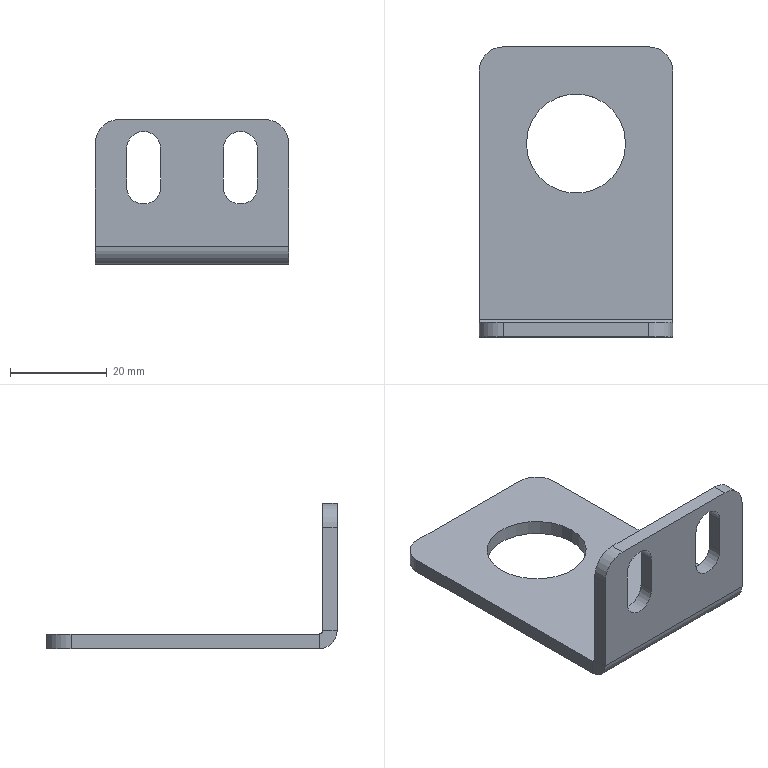Part | SolidWorks | features BaseBody 1 | 1 solid | 30 faces | box 40 x 60 x 30 mm | volume 8703 mm3 | plane 16 | cylinder 14 | commonest cylinder face diameters 7 x6 10 x4 20.5 x2 1.473 x1 7.473 x1
STEP:
#1=CARTESIAN_POINT('',(10.,-31.5,24.5));
#2=VERTEX_POINT('',#1);
#3=CARTESIAN_POINT('',(13.5,-31.5,21.));
#4=VERTEX_POINT('',#3);
#5=CARTESIAN_POINT('',(10.,-31.5,21.));
#6=DIRECTION('',(0.,1.,0.));
#7=DIRECTION('',(0.,0.,1.));
#8=AXIS2_PLACEMENT_3D('',#5,#6,#7);
#9=CIRCLE('',#8,3.5);
#10=EDGE_CURVE('',#2,#4,#9,.T.);
#11=ORIENTED_EDGE('',*,*,#10,.F.);
#12=CARTESIAN_POINT('',(10.,-28.5,24.5));
#13=VERTEX_POINT('',#12);
#14=CARTESIAN_POINT('',(10.,-38.5,24.5));
#15=DIRECTION('',(0.,1.,0.));
#16=VECTOR('',#15,1000.);
#17=LINE('',#14,#16);
#18=EDGE_CURVE('',#2,#13,#17,.T.);
#19=ORIENTED_EDGE('',*,*,#18,.T.);
#20=CARTESIAN_POINT('',(13.5,-28.5,21.));
#21=VERTEX_POINT('',#20);
#22=CARTESIAN_POINT('',(10.,-28.5,21.));
#23=DIRECTION('',(0.,1.,0.));
#24=DIRECTION('',(0.,0.,1.));
#25=AXIS2_PLACEMENT_3D('',#22,#23,#24);
#26=CIRCLE('',#25,3.5);
#27=EDGE_CURVE('',#13,#21,#26,.T.);
#28=ORIENTED_EDGE('',*,*,#27,.T.);
#29=CARTESIAN_POINT('',(13.5,-38.5,21.));
#30=DIRECTION('',(0.,1.,0.));
#31=VECTOR('',#30,1000.);
#32=LINE('',#29,#31);
#33=EDGE_CURVE('',#4,#21,#32,.T.);
#34=ORIENTED_EDGE('',*,*,#33,.F.);
#35=EDGE_LOOP('',(#11,#19,#28,#34));
#36=FACE_OUTER_BOUND('',#35,.T.);
#37=CARTESIAN_POINT('',(10.,-38.5,21.));
#38=DIRECTION('',(0.,1.,0.));
#39=DIRECTION('',(0.,0.,1.));
#40=AXIS2_PLACEMENT_3D('',#37,#38,#39);
#41=CYLINDRICAL_SURFACE('',#40,3.5);
#42=ADVANCED_FACE('',(#36),#41,.F.);
#43=CARTESIAN_POINT('',(-10.,-31.5,24.5));
#44=VERTEX_POINT('',#43);
#45=CARTESIAN_POINT('',(-6.5,-31.5,21.));
#46=VERTEX_POINT('',#45);
#47=CARTESIAN_POINT('',(-10.,-31.5,21.));
#48=DIRECTION('',(0.,1.,0.));
#49=DIRECTION('',(0.,0.,1.));
#50=AXIS2_PLACEMENT_3D('',#47,#48,#49);
#51=CIRCLE('',#50,3.5);
#52=EDGE_CURVE('',#44,#46,#51,.T.);
#53=ORIENTED_EDGE('',*,*,#52,.F.);
#54=CARTESIAN_POINT('',(-10.,-28.5,24.5));
#55=VERTEX_POINT('',#54);
#56=CARTESIAN_POINT('',(-10.,-38.5,24.5));
#57=DIRECTION('',(0.,1.,0.));
#58=VECTOR('',#57,1000.);
#59=LINE('',#56,#58);
#60=EDGE_CURVE('',#44,#55,#59,.T.);
#61=ORIENTED_EDGE('',*,*,#60,.T.);
#62=CARTESIAN_POINT('',(-6.5,-28.5,21.));
#63=VERTEX_POINT('',#62);
#64=CARTESIAN_POINT('',(-10.,-28.5,21.));
#65=DIRECTION('',(0.,1.,0.));
#66=DIRECTION('',(0.,0.,1.));
#67=AXIS2_PLACEMENT_3D('',#64,#65,#66);
#68=CIRCLE('',#67,3.5);
#69=EDGE_CURVE('',#55,#63,#68,.T.);
#70=ORIENTED_EDGE('',*,*,#69,.T.);
#71=CARTESIAN_POINT('',(-6.5,-38.5,21.));
#72=DIRECTION('',(0.,1.,0.));
#73=VECTOR('',#72,1000.);
#74=LINE('',#71,#73);
#75=EDGE_CURVE('',#46,#63,#74,.T.);
#76=ORIENTED_EDGE('',*,*,#75,.F.);
#77=EDGE_LOOP('',(#53,#61,#70,#76));
#78=FACE_OUTER_BOUND('',#77,.T.);
#79=CARTESIAN_POINT('',(-10.,-38.5,21.));
#80=DIRECTION('',(0.,1.,0.));
#81=DIRECTION('',(0.,0.,1.));
#82=AXIS2_PLACEMENT_3D('',#79,#80,#81);
#83=CYLINDRICAL_SURFACE('',#82,3.5);
#84=ADVANCED_FACE('',(#78),#83,.F.);
#85=CARTESIAN_POINT('',(-10.25,8.5,0.));
#86=VERTEX_POINT('',#85);
#87=CARTESIAN_POINT('',(10.25,8.5,0.));
#88=VERTEX_POINT('',#87);
#89=CARTESIAN_POINT('',(0.,8.5,0.));
#90=DIRECTION('',(0.,0.,1.));
#91=DIRECTION('',(1.,0.,0.));
#92=AXIS2_PLACEMENT_3D('',#89,#90,#91);
#93=CIRCLE('',#92,10.25);
#94=EDGE_CURVE('',#86,#88,#93,.T.);
#95=ORIENTED_EDGE('',*,*,#94,.T.);
#96=CARTESIAN_POINT('',(10.25,8.5,-3.));
#97=VERTEX_POINT('',#96);
#98=CARTESIAN_POINT('',(10.25,8.5,-3.));
#99=DIRECTION('',(0.,0.,-1.));
#100=VECTOR('',#99,1000.);
#101=LINE('',#98,#100);
#102=EDGE_CURVE('',#88,#97,#101,.T.);
#103=ORIENTED_EDGE('',*,*,#102,.T.);
#104=CARTESIAN_POINT('',(-10.25,8.5,-3.));
#105=VERTEX_POINT('',#104);
#106=CARTESIAN_POINT('',(0.,8.5,-3.));
#107=DIRECTION('',(0.,0.,-1.));
#108=DIRECTION('',(-1.,0.,0.));
#109=AXIS2_PLACEMENT_3D('',#106,#107,#108);
#110=CIRCLE('',#109,10.25);
#111=EDGE_CURVE('',#97,#105,#110,.T.);
#112=ORIENTED_EDGE('',*,*,#111,.T.);
#113=CARTESIAN_POINT('',(-10.25,8.5,-3.));
#114=DIRECTION('',(0.,0.,-1.));
#115=VECTOR('',#114,1000.);
#116=LINE('',#113,#115);
#117=EDGE_CURVE('',#86,#105,#116,.T.);
#118=ORIENTED_EDGE('',*,*,#117,.F.);
#119=EDGE_LOOP('',(#95,#103,#112,#118));
#120=FACE_OUTER_BOUND('',#119,.T.);
#121=CARTESIAN_POINT('',(0.,8.5,-3.));
#122=DIRECTION('',(0.,0.,-1.));
#123=DIRECTION('',(-1.,0.,0.));
#124=AXIS2_PLACEMENT_3D('',#121,#122,#123);
#125=CYLINDRICAL_SURFACE('',#124,10.25);
#126=ADVANCED_FACE('',(#120),#125,.F.);
#127=CARTESIAN_POINT('',(20.,-27.763,-3.));
#128=VERTEX_POINT('',#127);
#129=CARTESIAN_POINT('',(20.,23.5,-3.));
#130=VERTEX_POINT('',#129);
#131=CARTESIAN_POINT('',(20.,28.5,-3.));
#132=DIRECTION('',(0.,1.,0.));
#133=VECTOR('',#132,1000.);
#134=LINE('',#131,#133);
#135=EDGE_CURVE('',#128,#130,#134,.T.);
#136=ORIENTED_EDGE('',*,*,#135,.T.);
#137=CARTESIAN_POINT('',(20.,23.5,0.));
#138=VERTEX_POINT('',#137);
#139=CARTESIAN_POINT('',(20.,23.5,-3.));
#140=DIRECTION('',(0.,0.,1.));
#141=VECTOR('',#140,1000.);
#142=LINE('',#139,#141);
#143=EDGE_CURVE('',#130,#138,#142,.T.);
#144=ORIENTED_EDGE('',*,*,#143,.T.);
#145=CARTESIAN_POINT('',(20.,-27.763,0.));
#146=VERTEX_POINT('',#145);
#147=CARTESIAN_POINT('',(20.,28.5,0.));
#148=DIRECTION('',(0.,1.,0.));
#149=VECTOR('',#148,1000.);
#150=LINE('',#147,#149);
#151=EDGE_CURVE('',#146,#138,#150,.T.);
#152=ORIENTED_EDGE('',*,*,#151,.F.);
#153=CARTESIAN_POINT('',(20.,-27.763,0.));
#154=DIRECTION('',(0.,0.,-1.));
#155=VECTOR('',#154,1000.);
#156=LINE('',#153,#155);
#157=EDGE_CURVE('',#146,#128,#156,.T.);
#158=ORIENTED_EDGE('',*,*,#157,.T.);
#159=EDGE_LOOP('',(#136,#144,#152,#158));
#160=FACE_OUTER_BOUND('',#159,.T.);
#161=CARTESIAN_POINT('',(20.,28.5,-3.));
#162=DIRECTION('',(1.,0.,0.));
#163=DIRECTION('',(0.,1.,0.));
#164=AXIS2_PLACEMENT_3D('',#161,#162,#163);
#165=PLANE('',#164);
#166=ADVANCED_FACE('',(#160),#165,.T.);
#167=CARTESIAN_POINT('',(0.,8.5,-3.));
#168=DIRECTION('',(0.,0.,-1.));
#169=DIRECTION('',(-1.,0.,0.));
#170=AXIS2_PLACEMENT_3D('',#167,#168,#169);
#171=CIRCLE('',#170,10.25);
#172=EDGE_CURVE('',#105,#97,#171,.T.);
#173=ORIENTED_EDGE('',*,*,#172,.F.);
#174=ORIENTED_EDGE('',*,*,#111,.F.);
#175=EDGE_LOOP('',(#173,#174));
#176=FACE_BOUND('',#175,.T.);
#177=CARTESIAN_POINT('',(15.,28.5,-3.));
#178=VERTEX_POINT('',#177);
#179=CARTESIAN_POINT('',(-15.,28.5,-3.));
#180=VERTEX_POINT('',#179);
#181=CARTESIAN_POINT('',(-20.,28.5,-3.));
#182=DIRECTION('',(-1.,0.,0.));
#183=VECTOR('',#182,1000.);
#184=LINE('',#181,#183);
#185=EDGE_CURVE('',#178,#180,#184,.T.);
#186=ORIENTED_EDGE('',*,*,#185,.F.);
#187=CARTESIAN_POINT('',(15.,23.5,-3.));
#188=DIRECTION('',(0.,0.,-1.));
#189=DIRECTION('',(1.,0.,0.));
#190=AXIS2_PLACEMENT_3D('',#187,#188,#189);
#191=CIRCLE('',#190,5.);
#192=EDGE_CURVE('',#178,#130,#191,.T.);
#193=ORIENTED_EDGE('',*,*,#192,.T.);
#194=ORIENTED_EDGE('',*,*,#135,.F.);
#195=CARTESIAN_POINT('',(-20.,-27.763,-3.));
#196=VERTEX_POINT('',#195);
#197=CARTESIAN_POINT('',(20.,-27.763,-3.));
#198=DIRECTION('',(-1.,0.,0.));
#199=VECTOR('',#198,1000.);
#200=LINE('',#197,#199);
#201=EDGE_CURVE('',#128,#196,#200,.T.);
#202=ORIENTED_EDGE('',*,*,#201,.T.);
#203=CARTESIAN_POINT('',(-20.,23.5,-3.));
#204=VERTEX_POINT('',#203);
#205=CARTESIAN_POINT('',(-20.,28.5,-3.));
#206=DIRECTION('',(0.,-1.,0.));
#207=VECTOR('',#206,1000.);
#208=LINE('',#205,#207);
#209=EDGE_CURVE('',#204,#196,#208,.T.);
#210=ORIENTED_EDGE('',*,*,#209,.F.);
#211=CARTESIAN_POINT('',(-15.,23.5,-3.));
#212=DIRECTION('',(0.,0.,-1.));
#213=DIRECTION('',(1.,0.,0.));
#214=AXIS2_PLACEMENT_3D('',#211,#212,#213);
#215=CIRCLE('',#214,5.);
#216=EDGE_CURVE('',#204,#180,#215,.T.);
#217=ORIENTED_EDGE('',*,*,#216,.T.);
#218=EDGE_LOOP('',(#186,#193,#194,#202,#210,#217));
#219=FACE_OUTER_BOUND('',#218,.T.);
#220=CARTESIAN_POINT('',(0.,0.,-3.));
#221=DIRECTION('',(0.,0.,1.));
#222=DIRECTION('',(1.,0.,0.));
#223=AXIS2_PLACEMENT_3D('',#220,#221,#222);
#224=PLANE('',#223);
#225=ADVANCED_FACE('',(#176,#219),#224,.F.);
#226=ORIENTED_EDGE('',*,*,#94,.F.);
#227=CARTESIAN_POINT('',(0.,8.5,0.));
#228=DIRECTION('',(0.,0.,1.));
#229=DIRECTION('',(1.,0.,0.));
#230=AXIS2_PLACEMENT_3D('',#227,#228,#229);
#231=CIRCLE('',#230,10.25);
#232=EDGE_CURVE('',#88,#86,#231,.T.);
#233=ORIENTED_EDGE('',*,*,#232,.F.);
#234=EDGE_LOOP('',(#226,#233));
#235=FACE_BOUND('',#234,.T.);
#236=ORIENTED_EDGE('',*,*,#151,.T.);
#237=CARTESIAN_POINT('',(15.,28.5,0.));
#238=VERTEX_POINT('',#237);
#239=CARTESIAN_POINT('',(15.,23.5,0.));
#240=DIRECTION('',(0.,0.,1.));
#241=DIRECTION('',(1.,0.,0.));
#242=AXIS2_PLACEMENT_3D('',#239,#240,#241);
#243=CIRCLE('',#242,5.);
#244=EDGE_CURVE('',#138,#238,#243,.T.);
#245=ORIENTED_EDGE('',*,*,#244,.T.);
#246=CARTESIAN_POINT('',(-15.,28.5,0.));
#247=VERTEX_POINT('',#246);
#248=CARTESIAN_POINT('',(-20.,28.5,0.));
#249=DIRECTION('',(-1.,0.,0.));
#250=VECTOR('',#249,1000.);
#251=LINE('',#248,#250);
#252=EDGE_CURVE('',#238,#247,#251,.T.);
#253=ORIENTED_EDGE('',*,*,#252,.T.);
#254=CARTESIAN_POINT('',(-20.,23.5,0.));
#255=VERTEX_POINT('',#254);
#256=CARTESIAN_POINT('',(-15.,23.5,0.));
#257=DIRECTION('',(0.,0.,1.));
#258=DIRECTION('',(1.,0.,0.));
#259=AXIS2_PLACEMENT_3D('',#256,#257,#258);
#260=CIRCLE('',#259,5.);
#261=EDGE_CURVE('',#247,#255,#260,.T.);
#262=ORIENTED_EDGE('',*,*,#261,.T.);
#263=CARTESIAN_POINT('',(-20.,-27.763,0.));
#264=VERTEX_POINT('',#263);
#265=CARTESIAN_POINT('',(-20.,28.5,0.));
#266=DIRECTION('',(0.,-1.,0.));
#267=VECTOR('',#266,1000.);
#268=LINE('',#265,#267);
#269=EDGE_CURVE('',#255,#264,#268,.T.);
#270=ORIENTED_EDGE('',*,*,#269,.T.);
#271=CARTESIAN_POINT('',(20.,-27.763,0.));
#272=DIRECTION('',(-1.,0.,0.));
#273=VECTOR('',#272,1000.);
#274=LINE('',#271,#273);
#275=EDGE_CURVE('',#146,#264,#274,.T.);
#276=ORIENTED_EDGE('',*,*,#275,.F.);
#277=EDGE_LOOP('',(#236,#245,#253,#262,#270,#276));
#278=FACE_OUTER_BOUND('',#277,.T.);
#279=CARTESIAN_POINT('',(0.,0.,0.));
#280=DIRECTION('',(0.,0.,1.));
#281=DIRECTION('',(1.,0.,0.));
#282=AXIS2_PLACEMENT_3D('',#279,#280,#281);
#283=PLANE('',#282);
#284=ADVANCED_FACE('',(#235,#278),#283,.T.);
#285=ORIENTED_EDGE('',*,*,#269,.F.);
#286=CARTESIAN_POINT('',(-20.,23.5,-3.));
#287=DIRECTION('',(0.,0.,-1.));
#288=VECTOR('',#287,1000.);
#289=LINE('',#286,#288);
#290=EDGE_CURVE('',#255,#204,#289,.T.);
#291=ORIENTED_EDGE('',*,*,#290,.T.);
#292=ORIENTED_EDGE('',*,*,#209,.T.);
#293=CARTESIAN_POINT('',(-20.,-27.763,0.));
#294=DIRECTION('',(0.,0.,-1.));
#295=VECTOR('',#294,1000.);
#296=LINE('',#293,#295);
#297=EDGE_CURVE('',#264,#196,#296,.T.);
#298=ORIENTED_EDGE('',*,*,#297,.F.);
#299=EDGE_LOOP('',(#285,#291,#292,#298));
#300=FACE_OUTER_BOUND('',#299,.T.);
#301=CARTESIAN_POINT('',(-20.,28.5,-3.));
#302=DIRECTION('',(-1.,0.,0.));
#303=DIRECTION('',(0.,-1.,0.));
#304=AXIS2_PLACEMENT_3D('',#301,#302,#303);
#305=PLANE('',#304);
#306=ADVANCED_FACE('',(#300),#305,.T.);
#307=ORIENTED_EDGE('',*,*,#252,.F.);
#308=CARTESIAN_POINT('',(15.,28.5,-3.));
#309=DIRECTION('',(0.,0.,-1.));
#310=VECTOR('',#309,1000.);
#311=LINE('',#308,#310);
#312=EDGE_CURVE('',#238,#178,#311,.T.);
#313=ORIENTED_EDGE('',*,*,#312,.T.);
#314=ORIENTED_EDGE('',*,*,#185,.T.);
#315=CARTESIAN_POINT('',(-15.,28.5,-3.));
#316=DIRECTION('',(0.,0.,1.));
#317=VECTOR('',#316,1000.);
#318=LINE('',#315,#317);
#319=EDGE_CURVE('',#180,#247,#318,.T.);
#320=ORIENTED_EDGE('',*,*,#319,.T.);
#321=EDGE_LOOP('',(#307,#313,#314,#320));
#322=FACE_OUTER_BOUND('',#321,.T.);
#323=CARTESIAN_POINT('',(-20.,28.5,-3.));
#324=DIRECTION('',(0.,1.,0.));
#325=DIRECTION('',(0.,0.,1.));
#326=AXIS2_PLACEMENT_3D('',#323,#324,#325);
#327=PLANE('',#326);
#328=ADVANCED_FACE('',(#322),#327,.T.);
#329=CARTESIAN_POINT('',(-20.,-28.5,0.7366));
#330=VERTEX_POINT('',#329);
#331=CARTESIAN_POINT('',(-20.,-31.5,0.7366));
#332=VERTEX_POINT('',#331);
#333=CARTESIAN_POINT('',(-20.,-28.5,0.7366));
#334=DIRECTION('',(0.,-1.,0.));
#335=VECTOR('',#334,1000.);
#336=LINE('',#333,#335);
#337=EDGE_CURVE('',#330,#332,#336,.T.);
#338=ORIENTED_EDGE('',*,*,#337,.F.);
#339=CARTESIAN_POINT('',(-20.,-27.763,0.7366));
#340=DIRECTION('',(-1.,0.,0.));
#341=DIRECTION('',(0.,0.,-1.));
#342=AXIS2_PLACEMENT_3D('',#339,#340,#341);
#343=CIRCLE('',#342,0.7366);
#344=EDGE_CURVE('',#264,#330,#343,.T.);
#345=ORIENTED_EDGE('',*,*,#344,.F.);
#346=ORIENTED_EDGE('',*,*,#297,.T.);
#347=CARTESIAN_POINT('',(-20.,-27.763,0.7366));
#348=DIRECTION('',(-1.,0.,0.));
#349=DIRECTION('',(0.,0.,-1.));
#350=AXIS2_PLACEMENT_3D('',#347,#348,#349);
#351=CIRCLE('',#350,3.737);
#352=EDGE_CURVE('',#196,#332,#351,.T.);
#353=ORIENTED_EDGE('',*,*,#352,.T.);
#354=EDGE_LOOP('',(#338,#345,#346,#353));
#355=FACE_OUTER_BOUND('',#354,.T.);
#356=CARTESIAN_POINT('',(-20.,-27.763,0.7366));
#357=DIRECTION('',(-1.,0.,0.));
#358=DIRECTION('',(0.,0.,1.));
#359=AXIS2_PLACEMENT_3D('',#356,#357,#358);
#360=PLANE('',#359);
#361=ADVANCED_FACE('',(#355),#360,.T.);
#362=CARTESIAN_POINT('',(20.,-28.5,0.7366));
#363=VERTEX_POINT('',#362);
#364=CARTESIAN_POINT('',(20.,-27.763,0.7366));
#365=DIRECTION('',(1.,0.,0.));
#366=DIRECTION('',(0.,0.,-1.));
#367=AXIS2_PLACEMENT_3D('',#364,#365,#366);
#368=CIRCLE('',#367,0.7366);
#369=EDGE_CURVE('',#363,#146,#368,.T.);
#370=ORIENTED_EDGE('',*,*,#369,.F.);
#371=CARTESIAN_POINT('',(20.,-31.5,0.7366));
#372=VERTEX_POINT('',#371);
#373=CARTESIAN_POINT('',(20.,-28.5,0.7366));
#374=DIRECTION('',(0.,-1.,0.));
#375=VECTOR('',#374,1000.);
#376=LINE('',#373,#375);
#377=EDGE_CURVE('',#363,#372,#376,.T.);
#378=ORIENTED_EDGE('',*,*,#377,.T.);
#379=CARTESIAN_POINT('',(20.,-27.763,0.7366));
#380=DIRECTION('',(1.,0.,0.));
#381=DIRECTION('',(0.,0.,-1.));
#382=AXIS2_PLACEMENT_3D('',#379,#380,#381);
#383=CIRCLE('',#382,3.737);
#384=EDGE_CURVE('',#372,#128,#383,.T.);
#385=ORIENTED_EDGE('',*,*,#384,.T.);
#386=ORIENTED_EDGE('',*,*,#157,.F.);
#387=EDGE_LOOP('',(#370,#378,#385,#386));
#388=FACE_OUTER_BOUND('',#387,.T.);
#389=CARTESIAN_POINT('',(20.,-27.763,0.7366));
#390=DIRECTION('',(-1.,0.,0.));
#391=DIRECTION('',(0.,0.,1.));
#392=AXIS2_PLACEMENT_3D('',#389,#390,#391);
#393=PLANE('',#392);
#394=ADVANCED_FACE('',(#388),#393,.F.);
#395=ORIENTED_EDGE('',*,*,#201,.F.);
#396=ORIENTED_EDGE('',*,*,#384,.F.);
#397=CARTESIAN_POINT('',(0.,-31.5,0.7366));
#398=DIRECTION('',(-1.,0.,0.));
#399=VECTOR('',#398,1000.);
#400=LINE('',#397,#399);
#401=EDGE_CURVE('',#372,#332,#400,.T.);
#402=ORIENTED_EDGE('',*,*,#401,.T.);
#403=ORIENTED_EDGE('',*,*,#352,.F.);
#404=EDGE_LOOP('',(#395,#396,#402,#403));
#405=FACE_OUTER_BOUND('',#404,.T.);
#406=CARTESIAN_POINT('',(20.,-27.763,0.7366));
#407=DIRECTION('',(1.,0.,0.));
#408=DIRECTION('',(0.,-1.,0.));
#409=AXIS2_PLACEMENT_3D('',#406,#407,#408);
#410=CYLINDRICAL_SURFACE('',#409,3.737);
#411=ADVANCED_FACE('',(#405),#410,.T.);
#412=ORIENTED_EDGE('',*,*,#275,.T.);
#413=ORIENTED_EDGE('',*,*,#344,.T.);
#414=CARTESIAN_POINT('',(-20.,-28.5,0.7366));
#415=DIRECTION('',(1.,0.,0.));
#416=VECTOR('',#415,1000.);
#417=LINE('',#414,#416);
#418=EDGE_CURVE('',#330,#363,#417,.T.);
#419=ORIENTED_EDGE('',*,*,#418,.T.);
#420=ORIENTED_EDGE('',*,*,#369,.T.);
#421=EDGE_LOOP('',(#412,#413,#419,#420));
#422=FACE_OUTER_BOUND('',#421,.T.);
#423=CARTESIAN_POINT('',(20.,-27.763,0.7366));
#424=DIRECTION('',(1.,0.,0.));
#425=DIRECTION('',(0.,-1.,0.));
#426=AXIS2_PLACEMENT_3D('',#423,#424,#425);
#427=CYLINDRICAL_SURFACE('',#426,0.7366);
#428=ADVANCED_FACE('',(#422),#427,.F.);
#429=CARTESIAN_POINT('',(-20.,-31.5,22.));
#430=VERTEX_POINT('',#429);
#431=CARTESIAN_POINT('',(-20.,-31.5,0.));
#432=DIRECTION('',(0.,0.,-1.));
#433=VECTOR('',#432,1000.);
#434=LINE('',#431,#433);
#435=EDGE_CURVE('',#430,#332,#434,.T.);
#436=ORIENTED_EDGE('',*,*,#435,.F.);
#437=CARTESIAN_POINT('',(-20.,-28.5,22.));
#438=VERTEX_POINT('',#437);
#439=CARTESIAN_POINT('',(-20.,-31.5,22.));
#440=DIRECTION('',(0.,1.,0.));
#441=VECTOR('',#440,1000.);
#442=LINE('',#439,#441);
#443=EDGE_CURVE('',#430,#438,#442,.T.);
#444=ORIENTED_EDGE('',*,*,#443,.T.);
#445=CARTESIAN_POINT('',(-20.,-28.5,0.));
#446=DIRECTION('',(0.,0.,-1.));
#447=VECTOR('',#446,1000.);
#448=LINE('',#445,#447);
#449=EDGE_CURVE('',#438,#330,#448,.T.);
#450=ORIENTED_EDGE('',*,*,#449,.T.);
#451=ORIENTED_EDGE('',*,*,#337,.T.);
#452=EDGE_LOOP('',(#436,#444,#450,#451));
#453=FACE_OUTER_BOUND('',#452,.T.);
#454=CARTESIAN_POINT('',(-20.,-31.5,0.));
#455=DIRECTION('',(1.,0.,0.));
#456=DIRECTION('',(0.,0.,-1.));
#457=AXIS2_PLACEMENT_3D('',#454,#455,#456);
#458=PLANE('',#457);
#459=ADVANCED_FACE('',(#453),#458,.F.);
#460=CARTESIAN_POINT('',(20.,-28.5,22.));
#461=VERTEX_POINT('',#460);
#462=CARTESIAN_POINT('',(20.,-28.5,27.));
#463=DIRECTION('',(0.,0.,1.));
#464=VECTOR('',#463,1000.);
#465=LINE('',#462,#464);
#466=EDGE_CURVE('',#363,#461,#465,.T.);
#467=ORIENTED_EDGE('',*,*,#466,.T.);
#468=CARTESIAN_POINT('',(20.,-31.5,22.));
#469=VERTEX_POINT('',#468);
#470=CARTESIAN_POINT('',(20.,-31.5,22.));
#471=DIRECTION('',(0.,-1.,0.));
#472=VECTOR('',#471,1000.);
#473=LINE('',#470,#472);
#474=EDGE_CURVE('',#461,#469,#473,.T.);
#475=ORIENTED_EDGE('',*,*,#474,.T.);
#476=CARTESIAN_POINT('',(20.,-31.5,27.));
#477=DIRECTION('',(0.,0.,1.));
#478=VECTOR('',#477,1000.);
#479=LINE('',#476,#478);
#480=EDGE_CURVE('',#372,#469,#479,.T.);
#481=ORIENTED_EDGE('',*,*,#480,.F.);
#482=ORIENTED_EDGE('',*,*,#377,.F.);
#483=EDGE_LOOP('',(#467,#475,#481,#482));
#484=FACE_OUTER_BOUND('',#483,.T.);
#485=CARTESIAN_POINT('',(20.,-31.5,27.));
#486=DIRECTION('',(-1.,0.,0.));
#487=DIRECTION('',(0.,0.,1.));
#488=AXIS2_PLACEMENT_3D('',#485,#486,#487);
#489=PLANE('',#488);
#490=ADVANCED_FACE('',(#484),#489,.F.);
#491=CARTESIAN_POINT('',(13.5,-31.5,13.));
#492=VERTEX_POINT('',#491);
#493=CARTESIAN_POINT('',(13.5,-31.5,0.));
#494=DIRECTION('',(0.,0.,-1.));
#495=VECTOR('',#494,1000.);
#496=LINE('',#493,#495);
#497=EDGE_CURVE('',#4,#492,#496,.T.);
#498=ORIENTED_EDGE('',*,*,#497,.T.);
#499=CARTESIAN_POINT('',(6.5,-31.5,13.));
#500=VERTEX_POINT('',#499);
#501=CARTESIAN_POINT('',(10.,-31.5,13.));
#502=DIRECTION('',(0.,1.,0.));
#503=DIRECTION('',(0.,0.,1.));
#504=AXIS2_PLACEMENT_3D('',#501,#502,#503);
#505=CIRCLE('',#504,3.5);
#506=EDGE_CURVE('',#492,#500,#505,.T.);
#507=ORIENTED_EDGE('',*,*,#506,.T.);
#508=CARTESIAN_POINT('',(6.5,-31.5,21.));
#509=VERTEX_POINT('',#508);
#510=CARTESIAN_POINT('',(6.5,-31.5,0.));
#511=DIRECTION('',(0.,0.,1.));
#512=VECTOR('',#511,1000.);
#513=LINE('',#510,#512);
#514=EDGE_CURVE('',#500,#509,#513,.T.);
#515=ORIENTED_EDGE('',*,*,#514,.T.);
#516=CARTESIAN_POINT('',(10.,-31.5,21.));
#517=DIRECTION('',(0.,1.,0.));
#518=DIRECTION('',(0.,0.,1.));
#519=AXIS2_PLACEMENT_3D('',#516,#517,#518);
#520=CIRCLE('',#519,3.5);
#521=EDGE_CURVE('',#509,#2,#520,.T.);
#522=ORIENTED_EDGE('',*,*,#521,.T.);
#523=ORIENTED_EDGE('',*,*,#10,.T.);
#524=EDGE_LOOP('',(#498,#507,#515,#522,#523));
#525=FACE_BOUND('',#524,.T.);
#526=CARTESIAN_POINT('',(-6.5,-31.5,13.));
#527=VERTEX_POINT('',#526);
#528=CARTESIAN_POINT('',(-6.5,-31.5,0.));
#529=DIRECTION('',(0.,0.,-1.));
#530=VECTOR('',#529,1000.);
#531=LINE('',#528,#530);
#532=EDGE_CURVE('',#46,#527,#531,.T.);
#533=ORIENTED_EDGE('',*,*,#532,.T.);
#534=CARTESIAN_POINT('',(-13.5,-31.5,13.));
#535=VERTEX_POINT('',#534);
#536=CARTESIAN_POINT('',(-10.,-31.5,13.));
#537=DIRECTION('',(0.,1.,0.));
#538=DIRECTION('',(0.,0.,1.));
#539=AXIS2_PLACEMENT_3D('',#536,#537,#538);
#540=CIRCLE('',#539,3.5);
#541=EDGE_CURVE('',#527,#535,#540,.T.);
#542=ORIENTED_EDGE('',*,*,#541,.T.);
#543=CARTESIAN_POINT('',(-13.5,-31.5,21.));
#544=VERTEX_POINT('',#543);
#545=CARTESIAN_POINT('',(-13.5,-31.5,0.));
#546=DIRECTION('',(0.,0.,1.));
#547=VECTOR('',#546,1000.);
#548=LINE('',#545,#547);
#549=EDGE_CURVE('',#535,#544,#548,.T.);
#550=ORIENTED_EDGE('',*,*,#549,.T.);
#551=CARTESIAN_POINT('',(-10.,-31.5,21.));
#552=DIRECTION('',(0.,1.,0.));
#553=DIRECTION('',(0.,0.,1.));
#554=AXIS2_PLACEMENT_3D('',#551,#552,#553);
#555=CIRCLE('',#554,3.5);
#556=EDGE_CURVE('',#544,#44,#555,.T.);
#557=ORIENTED_EDGE('',*,*,#556,.T.);
#558=ORIENTED_EDGE('',*,*,#52,.T.);
#559=EDGE_LOOP('',(#533,#542,#550,#557,#558));
#560=FACE_BOUND('',#559,.T.);
#561=CARTESIAN_POINT('',(15.,-31.5,27.));
#562=VERTEX_POINT('',#561);
#563=CARTESIAN_POINT('',(-15.,-31.5,27.));
#564=VERTEX_POINT('',#563);
#565=CARTESIAN_POINT('',(-20.,-31.5,27.));
#566=DIRECTION('',(-1.,0.,0.));
#567=VECTOR('',#566,1000.);
#568=LINE('',#565,#567);
#569=EDGE_CURVE('',#562,#564,#568,.T.);
#570=ORIENTED_EDGE('',*,*,#569,.T.);
#571=CARTESIAN_POINT('',(-15.,-31.5,22.));
#572=DIRECTION('',(0.,-1.,0.));
#573=DIRECTION('',(0.,0.,1.));
#574=AXIS2_PLACEMENT_3D('',#571,#572,#573);
#575=CIRCLE('',#574,5.);
#576=EDGE_CURVE('',#564,#430,#575,.T.);
#577=ORIENTED_EDGE('',*,*,#576,.T.);
#578=ORIENTED_EDGE('',*,*,#435,.T.);
#579=ORIENTED_EDGE('',*,*,#401,.F.);
#580=ORIENTED_EDGE('',*,*,#480,.T.);
#581=CARTESIAN_POINT('',(15.,-31.5,22.));
#582=DIRECTION('',(0.,-1.,0.));
#583=DIRECTION('',(0.,0.,1.));
#584=AXIS2_PLACEMENT_3D('',#581,#582,#583);
#585=CIRCLE('',#584,5.);
#586=EDGE_CURVE('',#469,#562,#585,.T.);
#587=ORIENTED_EDGE('',*,*,#586,.T.);
#588=EDGE_LOOP('',(#570,#577,#578,#579,#580,#587));
#589=FACE_OUTER_BOUND('',#588,.T.);
#590=CARTESIAN_POINT('',(0.,-31.5,0.));
#591=DIRECTION('',(0.,1.,0.));
#592=DIRECTION('',(0.,0.,1.));
#593=AXIS2_PLACEMENT_3D('',#590,#591,#592);
#594=PLANE('',#593);
#595=ADVANCED_FACE('',(#525,#560,#589),#594,.F.);
#596=CARTESIAN_POINT('',(13.5,-28.5,13.));
#597=VERTEX_POINT('',#596);
#598=CARTESIAN_POINT('',(6.5,-28.5,13.));
#599=VERTEX_POINT('',#598);
#600=CARTESIAN_POINT('',(10.,-28.5,13.));
#601=DIRECTION('',(0.,1.,0.));
#602=DIRECTION('',(0.,0.,1.));
#603=AXIS2_PLACEMENT_3D('',#600,#601,#602);
#604=CIRCLE('',#603,3.5);
#605=EDGE_CURVE('',#597,#599,#604,.T.);
#606=ORIENTED_EDGE('',*,*,#605,.F.);
#607=CARTESIAN_POINT('',(13.5,-28.5,13.));
#608=DIRECTION('',(0.,0.,-1.));
#609=VECTOR('',#608,1000.);
#610=LINE('',#607,#609);
#611=EDGE_CURVE('',#21,#597,#610,.T.);
#612=ORIENTED_EDGE('',*,*,#611,.F.);
#613=ORIENTED_EDGE('',*,*,#27,.F.);
#614=CARTESIAN_POINT('',(6.5,-28.5,21.));
#615=VERTEX_POINT('',#614);
#616=CARTESIAN_POINT('',(10.,-28.5,21.));
#617=DIRECTION('',(0.,1.,0.));
#618=DIRECTION('',(0.,0.,1.));
#619=AXIS2_PLACEMENT_3D('',#616,#617,#618);
#620=CIRCLE('',#619,3.5);
#621=EDGE_CURVE('',#615,#13,#620,.T.);
#622=ORIENTED_EDGE('',*,*,#621,.F.);
#623=CARTESIAN_POINT('',(6.5,-28.5,13.));
#624=DIRECTION('',(0.,0.,1.));
#625=VECTOR('',#624,1000.);
#626=LINE('',#623,#625);
#627=EDGE_CURVE('',#599,#615,#626,.T.);
#628=ORIENTED_EDGE('',*,*,#627,.F.);
#629=EDGE_LOOP('',(#606,#612,#613,#622,#628));
#630=FACE_BOUND('',#629,.T.);
#631=CARTESIAN_POINT('',(-6.5,-28.5,13.));
#632=VERTEX_POINT('',#631);
#633=CARTESIAN_POINT('',(-13.5,-28.5,13.));
#634=VERTEX_POINT('',#633);
#635=CARTESIAN_POINT('',(-10.,-28.5,13.));
#636=DIRECTION('',(0.,1.,0.));
#637=DIRECTION('',(0.,0.,1.));
#638=AXIS2_PLACEMENT_3D('',#635,#636,#637);
#639=CIRCLE('',#638,3.5);
#640=EDGE_CURVE('',#632,#634,#639,.T.);
#641=ORIENTED_EDGE('',*,*,#640,.F.);
#642=CARTESIAN_POINT('',(-6.5,-28.5,13.));
#643=DIRECTION('',(0.,0.,-1.));
#644=VECTOR('',#643,1000.);
#645=LINE('',#642,#644);
#646=EDGE_CURVE('',#63,#632,#645,.T.);
#647=ORIENTED_EDGE('',*,*,#646,.F.);
#648=ORIENTED_EDGE('',*,*,#69,.F.);
#649=CARTESIAN_POINT('',(-13.5,-28.5,21.));
#650=VERTEX_POINT('',#649);
#651=CARTESIAN_POINT('',(-10.,-28.5,21.));
#652=DIRECTION('',(0.,1.,0.));
#653=DIRECTION('',(0.,0.,1.));
#654=AXIS2_PLACEMENT_3D('',#651,#652,#653);
#655=CIRCLE('',#654,3.5);
#656=EDGE_CURVE('',#650,#55,#655,.T.);
#657=ORIENTED_EDGE('',*,*,#656,.F.);
#658=CARTESIAN_POINT('',(-13.5,-28.5,13.));
#659=DIRECTION('',(0.,0.,1.));
#660=VECTOR('',#659,1000.);
#661=LINE('',#658,#660);
#662=EDGE_CURVE('',#634,#650,#661,.T.);
#663=ORIENTED_EDGE('',*,*,#662,.F.);
#664=EDGE_LOOP('',(#641,#647,#648,#657,#663));
#665=FACE_BOUND('',#664,.T.);
#666=ORIENTED_EDGE('',*,*,#449,.F.);
#667=CARTESIAN_POINT('',(-15.,-28.5,27.));
#668=VERTEX_POINT('',#667);
#669=CARTESIAN_POINT('',(-15.,-28.5,22.));
#670=DIRECTION('',(0.,1.,0.));
#671=DIRECTION('',(0.,0.,1.));
#672=AXIS2_PLACEMENT_3D('',#669,#670,#671);
#673=CIRCLE('',#672,5.);
#674=EDGE_CURVE('',#438,#668,#673,.T.);
#675=ORIENTED_EDGE('',*,*,#674,.T.);
#676=CARTESIAN_POINT('',(15.,-28.5,27.));
#677=VERTEX_POINT('',#676);
#678=CARTESIAN_POINT('',(-20.,-28.5,27.));
#679=DIRECTION('',(-1.,0.,0.));
#680=VECTOR('',#679,1000.);
#681=LINE('',#678,#680);
#682=EDGE_CURVE('',#677,#668,#681,.T.);
#683=ORIENTED_EDGE('',*,*,#682,.F.);
#684=CARTESIAN_POINT('',(15.,-28.5,22.));
#685=DIRECTION('',(0.,1.,0.));
#686=DIRECTION('',(0.,0.,1.));
#687=AXIS2_PLACEMENT_3D('',#684,#685,#686);
#688=CIRCLE('',#687,5.);
#689=EDGE_CURVE('',#677,#461,#688,.T.);
#690=ORIENTED_EDGE('',*,*,#689,.T.);
#691=ORIENTED_EDGE('',*,*,#466,.F.);
#692=ORIENTED_EDGE('',*,*,#418,.F.);
#693=EDGE_LOOP('',(#666,#675,#683,#690,#691,#692));
#694=FACE_OUTER_BOUND('',#693,.T.);
#695=CARTESIAN_POINT('',(0.,-28.5,0.));
#696=DIRECTION('',(0.,1.,0.));
#697=DIRECTION('',(0.,0.,1.));
#698=AXIS2_PLACEMENT_3D('',#695,#696,#697);
#699=PLANE('',#698);
#700=ADVANCED_FACE('',(#630,#665,#694),#699,.T.);
#701=ORIENTED_EDGE('',*,*,#682,.T.);
#702=CARTESIAN_POINT('',(-15.,-31.5,27.));
#703=DIRECTION('',(0.,-1.,0.));
#704=VECTOR('',#703,1000.);
#705=LINE('',#702,#704);
#706=EDGE_CURVE('',#668,#564,#705,.T.);
#707=ORIENTED_EDGE('',*,*,#706,.T.);
#708=ORIENTED_EDGE('',*,*,#569,.F.);
#709=CARTESIAN_POINT('',(15.,-31.5,27.));
#710=DIRECTION('',(0.,1.,0.));
#711=VECTOR('',#710,1000.);
#712=LINE('',#709,#711);
#713=EDGE_CURVE('',#562,#677,#712,.T.);
#714=ORIENTED_EDGE('',*,*,#713,.T.);
#715=EDGE_LOOP('',(#701,#707,#708,#714));
#716=FACE_OUTER_BOUND('',#715,.T.);
#717=CARTESIAN_POINT('',(-20.,-31.5,27.));
#718=DIRECTION('',(0.,0.,-1.));
#719=DIRECTION('',(0.,1.,0.));
#720=AXIS2_PLACEMENT_3D('',#717,#718,#719);
#721=PLANE('',#720);
#722=ADVANCED_FACE('',(#716),#721,.F.);
#723=ORIENTED_EDGE('',*,*,#102,.F.);
#724=ORIENTED_EDGE('',*,*,#232,.T.);
#725=ORIENTED_EDGE('',*,*,#117,.T.);
#726=ORIENTED_EDGE('',*,*,#172,.T.);
#727=EDGE_LOOP('',(#723,#724,#725,#726));
#728=FACE_OUTER_BOUND('',#727,.T.);
#729=CARTESIAN_POINT('',(0.,8.5,-3.));
#730=DIRECTION('',(0.,0.,-1.));
#731=DIRECTION('',(-1.,0.,0.));
#732=AXIS2_PLACEMENT_3D('',#729,#730,#731);
#733=CYLINDRICAL_SURFACE('',#732,10.25);
#734=ADVANCED_FACE('',(#728),#733,.F.);
#735=ORIENTED_EDGE('',*,*,#576,.F.);
#736=ORIENTED_EDGE('',*,*,#706,.F.);
#737=ORIENTED_EDGE('',*,*,#674,.F.);
#738=ORIENTED_EDGE('',*,*,#443,.F.);
#739=EDGE_LOOP('',(#735,#736,#737,#738));
#740=FACE_OUTER_BOUND('',#739,.T.);
#741=CARTESIAN_POINT('',(-15.,-31.5,22.));
#742=DIRECTION('',(0.,1.,0.));
#743=DIRECTION('',(0.,0.,1.));
#744=AXIS2_PLACEMENT_3D('',#741,#742,#743);
#745=CYLINDRICAL_SURFACE('',#744,5.);
#746=ADVANCED_FACE('',(#740),#745,.T.);
#747=ORIENTED_EDGE('',*,*,#586,.F.);
#748=ORIENTED_EDGE('',*,*,#474,.F.);
#749=ORIENTED_EDGE('',*,*,#689,.F.);
#750=ORIENTED_EDGE('',*,*,#713,.F.);
#751=EDGE_LOOP('',(#747,#748,#749,#750));
#752=FACE_OUTER_BOUND('',#751,.T.);
#753=CARTESIAN_POINT('',(15.,-31.5,22.));
#754=DIRECTION('',(0.,1.,0.));
#755=DIRECTION('',(0.,0.,1.));
#756=AXIS2_PLACEMENT_3D('',#753,#754,#755);
#757=CYLINDRICAL_SURFACE('',#756,5.);
#758=ADVANCED_FACE('',(#752),#757,.T.);
#759=ORIENTED_EDGE('',*,*,#192,.F.);
#760=ORIENTED_EDGE('',*,*,#312,.F.);
#761=ORIENTED_EDGE('',*,*,#244,.F.);
#762=ORIENTED_EDGE('',*,*,#143,.F.);
#763=EDGE_LOOP('',(#759,#760,#761,#762));
#764=FACE_OUTER_BOUND('',#763,.T.);
#765=CARTESIAN_POINT('',(15.,23.5,-3.));
#766=DIRECTION('',(0.,0.,1.));
#767=DIRECTION('',(1.,0.,0.));
#768=AXIS2_PLACEMENT_3D('',#765,#766,#767);
#769=CYLINDRICAL_SURFACE('',#768,5.);
#770=ADVANCED_FACE('',(#764),#769,.T.);
#771=ORIENTED_EDGE('',*,*,#216,.F.);
#772=ORIENTED_EDGE('',*,*,#290,.F.);
#773=ORIENTED_EDGE('',*,*,#261,.F.);
#774=ORIENTED_EDGE('',*,*,#319,.F.);
#775=EDGE_LOOP('',(#771,#772,#773,#774));
#776=FACE_OUTER_BOUND('',#775,.T.);
#777=CARTESIAN_POINT('',(-15.,23.5,-3.));
#778=DIRECTION('',(0.,0.,1.));
#779=DIRECTION('',(1.,0.,0.));
#780=AXIS2_PLACEMENT_3D('',#777,#778,#779);
#781=CYLINDRICAL_SURFACE('',#780,5.);
#782=ADVANCED_FACE('',(#776),#781,.T.);
#783=CARTESIAN_POINT('',(-6.5,-38.5,13.));
#784=DIRECTION('',(0.,1.,0.));
#785=VECTOR('',#784,1000.);
#786=LINE('',#783,#785);
#787=EDGE_CURVE('',#527,#632,#786,.T.);
#788=ORIENTED_EDGE('',*,*,#787,.T.);
#789=ORIENTED_EDGE('',*,*,#640,.T.);
#790=CARTESIAN_POINT('',(-13.5,-38.5,13.));
#791=DIRECTION('',(0.,1.,0.));
#792=VECTOR('',#791,1000.);
#793=LINE('',#790,#792);
#794=EDGE_CURVE('',#535,#634,#793,.T.);
#795=ORIENTED_EDGE('',*,*,#794,.F.);
#796=ORIENTED_EDGE('',*,*,#541,.F.);
#797=EDGE_LOOP('',(#788,#789,#795,#796));
#798=FACE_OUTER_BOUND('',#797,.T.);
#799=CARTESIAN_POINT('',(-10.,-38.5,13.));
#800=DIRECTION('',(0.,1.,0.));
#801=DIRECTION('',(0.,0.,1.));
#802=AXIS2_PLACEMENT_3D('',#799,#800,#801);
#803=CYLINDRICAL_SURFACE('',#802,3.5);
#804=ADVANCED_FACE('',(#798),#803,.F.);
#805=ORIENTED_EDGE('',*,*,#75,.T.);
#806=ORIENTED_EDGE('',*,*,#646,.T.);
#807=ORIENTED_EDGE('',*,*,#787,.F.);
#808=ORIENTED_EDGE('',*,*,#532,.F.);
#809=EDGE_LOOP('',(#805,#806,#807,#808));
#810=FACE_OUTER_BOUND('',#809,.T.);
#811=CARTESIAN_POINT('',(-6.5,-38.5,13.));
#812=DIRECTION('',(1.,0.,0.));
#813=DIRECTION('',(0.,0.,-1.));
#814=AXIS2_PLACEMENT_3D('',#811,#812,#813);
#815=PLANE('',#814);
#816=ADVANCED_FACE('',(#810),#815,.F.);
#817=ORIENTED_EDGE('',*,*,#60,.F.);
#818=ORIENTED_EDGE('',*,*,#556,.F.);
#819=CARTESIAN_POINT('',(-13.5,-38.5,21.));
#820=DIRECTION('',(0.,1.,0.));
#821=VECTOR('',#820,1000.);
#822=LINE('',#819,#821);
#823=EDGE_CURVE('',#544,#650,#822,.T.);
#824=ORIENTED_EDGE('',*,*,#823,.T.);
#825=ORIENTED_EDGE('',*,*,#656,.T.);
#826=EDGE_LOOP('',(#817,#818,#824,#825));
#827=FACE_OUTER_BOUND('',#826,.T.);
#828=CARTESIAN_POINT('',(-10.,-38.5,21.));
#829=DIRECTION('',(0.,1.,0.));
#830=DIRECTION('',(0.,0.,1.));
#831=AXIS2_PLACEMENT_3D('',#828,#829,#830);
#832=CYLINDRICAL_SURFACE('',#831,3.5);
#833=ADVANCED_FACE('',(#827),#832,.F.);
#834=ORIENTED_EDGE('',*,*,#794,.T.);
#835=ORIENTED_EDGE('',*,*,#662,.T.);
#836=ORIENTED_EDGE('',*,*,#823,.F.);
#837=ORIENTED_EDGE('',*,*,#549,.F.);
#838=EDGE_LOOP('',(#834,#835,#836,#837));
#839=FACE_OUTER_BOUND('',#838,.T.);
#840=CARTESIAN_POINT('',(-13.5,-38.5,13.));
#841=DIRECTION('',(-1.,0.,0.));
#842=DIRECTION('',(0.,0.,1.));
#843=AXIS2_PLACEMENT_3D('',#840,#841,#842);
#844=PLANE('',#843);
#845=ADVANCED_FACE('',(#839),#844,.F.);
#846=CARTESIAN_POINT('',(13.5,-38.5,13.));
#847=DIRECTION('',(0.,1.,0.));
#848=VECTOR('',#847,1000.);
#849=LINE('',#846,#848);
#850=EDGE_CURVE('',#492,#597,#849,.T.);
#851=ORIENTED_EDGE('',*,*,#850,.T.);
#852=ORIENTED_EDGE('',*,*,#605,.T.);
#853=CARTESIAN_POINT('',(6.5,-38.5,13.));
#854=DIRECTION('',(0.,1.,0.));
#855=VECTOR('',#854,1000.);
#856=LINE('',#853,#855);
#857=EDGE_CURVE('',#500,#599,#856,.T.);
#858=ORIENTED_EDGE('',*,*,#857,.F.);
#859=ORIENTED_EDGE('',*,*,#506,.F.);
#860=EDGE_LOOP('',(#851,#852,#858,#859));
#861=FACE_OUTER_BOUND('',#860,.T.);
#862=CARTESIAN_POINT('',(10.,-38.5,13.));
#863=DIRECTION('',(0.,1.,0.));
#864=DIRECTION('',(0.,0.,1.));
#865=AXIS2_PLACEMENT_3D('',#862,#863,#864);
#866=CYLINDRICAL_SURFACE('',#865,3.5);
#867=ADVANCED_FACE('',(#861),#866,.F.);
#868=ORIENTED_EDGE('',*,*,#33,.T.);
#869=ORIENTED_EDGE('',*,*,#611,.T.);
#870=ORIENTED_EDGE('',*,*,#850,.F.);
#871=ORIENTED_EDGE('',*,*,#497,.F.);
#872=EDGE_LOOP('',(#868,#869,#870,#871));
#873=FACE_OUTER_BOUND('',#872,.T.);
#874=CARTESIAN_POINT('',(13.5,-38.5,13.));
#875=DIRECTION('',(1.,0.,0.));
#876=DIRECTION('',(0.,0.,-1.));
#877=AXIS2_PLACEMENT_3D('',#874,#875,#876);
#878=PLANE('',#877);
#879=ADVANCED_FACE('',(#873),#878,.F.);
#880=ORIENTED_EDGE('',*,*,#18,.F.);
#881=ORIENTED_EDGE('',*,*,#521,.F.);
#882=CARTESIAN_POINT('',(6.5,-38.5,21.));
#883=DIRECTION('',(0.,1.,0.));
#884=VECTOR('',#883,1000.);
#885=LINE('',#882,#884);
#886=EDGE_CURVE('',#509,#615,#885,.T.);
#887=ORIENTED_EDGE('',*,*,#886,.T.);
#888=ORIENTED_EDGE('',*,*,#621,.T.);
#889=EDGE_LOOP('',(#880,#881,#887,#888));
#890=FACE_OUTER_BOUND('',#889,.T.);
#891=CARTESIAN_POINT('',(10.,-38.5,21.));
#892=DIRECTION('',(0.,1.,0.));
#893=DIRECTION('',(0.,0.,1.));
#894=AXIS2_PLACEMENT_3D('',#891,#892,#893);
#895=CYLINDRICAL_SURFACE('',#894,3.5);
#896=ADVANCED_FACE('',(#890),#895,.F.);
#897=ORIENTED_EDGE('',*,*,#857,.T.);
#898=ORIENTED_EDGE('',*,*,#627,.T.);
#899=ORIENTED_EDGE('',*,*,#886,.F.);
#900=ORIENTED_EDGE('',*,*,#514,.F.);
#901=EDGE_LOOP('',(#897,#898,#899,#900));
#902=FACE_OUTER_BOUND('',#901,.T.);
#903=CARTESIAN_POINT('',(6.5,-38.5,13.));
#904=DIRECTION('',(-1.,0.,0.));
#905=DIRECTION('',(0.,0.,1.));
#906=AXIS2_PLACEMENT_3D('',#903,#904,#905);
#907=PLANE('',#906);
#908=ADVANCED_FACE('',(#902),#907,.F.);
#909=CLOSED_SHELL('',(#42,#84,#126,#166,#225,#284,#306,#328,#361,#394,#411,#428,#459,#490,#595,#700,#722,#734,#746,#758,#770,#782,#804,#816,#833,#845,#867,#879,#896,#908));
#910=MANIFOLD_SOLID_BREP('',#909);
#911=CARTESIAN_POINT('',(0.,0.,0.));
#912=DIRECTION('',(0.,0.,1.));
#913=DIRECTION('',(1.,0.,0.));
#914=AXIS2_PLACEMENT_3D('',#911,#912,#913);
#915=(LENGTH_UNIT()NAMED_UNIT(*)SI_UNIT(.MILLI.,.METRE.));
#916=UNCERTAINTY_MEASURE_WITH_UNIT(LENGTH_MEASURE(0.00001),#915,'','');
#917=(NAMED_UNIT(*)PLANE_ANGLE_UNIT()SI_UNIT($,.RADIAN.));
#918=(NAMED_UNIT(*)SI_UNIT($,.STERADIAN.)SOLID_ANGLE_UNIT());
#919=(GEOMETRIC_REPRESENTATION_CONTEXT(3)GLOBAL_UNCERTAINTY_ASSIGNED_CONTEXT((#916))GLOBAL_UNIT_ASSIGNED_CONTEXT((#915,#917,#918))REPRESENTATION_CONTEXT('',''));
#920=ADVANCED_BREP_SHAPE_REPRESENTATION('',(#910,#914),#919);